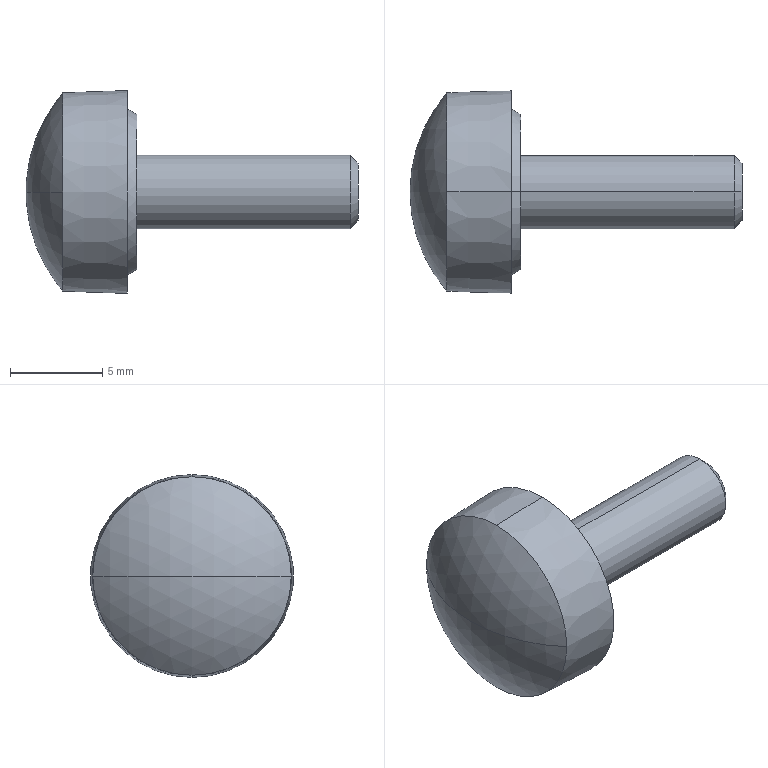Part | SolidWorks | features BaseBody 1 | 1 solid | 13 faces | box 18 x 11 x 11 mm | volume 599.857 mm3 | cone 6 | plane 3 | sphere 2 | cylinder 2 | commonest cylinder face diameters 4 x2
STEP:
#1=CARTESIAN_POINT('',(-4.,5.378,0.));
#2=VERTEX_POINT('',#1);
#3=CARTESIAN_POINT('',(-4.,-5.378,0.));
#4=VERTEX_POINT('',#3);
#5=CARTESIAN_POINT('',(2.23,0.,0.));
#6=DIRECTION('',(0.,0.,1.));
#7=DIRECTION('',(-0.757,0.6534,0.));
#8=AXIS2_PLACEMENT_3D('',#5,#6,#7);
#9=CIRCLE('',#8,8.23);
#10=EDGE_CURVE('',#2,#4,#9,.T.);
#11=ORIENTED_EDGE('',*,*,#10,.F.);
#12=CARTESIAN_POINT('',(-4.,0.,-5.378));
#13=VERTEX_POINT('',#12);
#14=CARTESIAN_POINT('',(-4.,0.,0.));
#15=DIRECTION('',(1.,0.,0.));
#16=DIRECTION('',(0.,0.,-1.));
#17=AXIS2_PLACEMENT_3D('',#14,#15,#16);
#18=CIRCLE('',#17,5.378);
#19=EDGE_CURVE('',#13,#2,#18,.T.);
#20=ORIENTED_EDGE('',*,*,#19,.F.);
#21=CARTESIAN_POINT('',(-4.,0.,0.));
#22=DIRECTION('',(1.,0.,0.));
#23=DIRECTION('',(0.,0.,-1.));
#24=AXIS2_PLACEMENT_3D('',#21,#22,#23);
#25=CIRCLE('',#24,5.378);
#26=EDGE_CURVE('',#4,#13,#25,.T.);
#27=ORIENTED_EDGE('',*,*,#26,.F.);
#28=EDGE_LOOP('',(#11,#20,#27));
#29=FACE_OUTER_BOUND('',#28,.T.);
#30=CARTESIAN_POINT('',(2.23,0.,0.));
#31=DIRECTION('',(0.,-1.,0.));
#32=DIRECTION('',(0.,0.,1.));
#33=AXIS2_PLACEMENT_3D('',#30,#31,#32);
#34=SPHERICAL_SURFACE('',#33,8.23);
#35=ADVANCED_FACE('',(#29),#34,.T.);
#36=ORIENTED_EDGE('',*,*,#10,.T.);
#37=CARTESIAN_POINT('',(-4.,0.,5.378));
#38=VERTEX_POINT('',#37);
#39=CARTESIAN_POINT('',(-4.,0.,0.));
#40=DIRECTION('',(1.,0.,0.));
#41=DIRECTION('',(0.,0.,-1.));
#42=AXIS2_PLACEMENT_3D('',#39,#40,#41);
#43=CIRCLE('',#42,5.378);
#44=EDGE_CURVE('',#38,#4,#43,.T.);
#45=ORIENTED_EDGE('',*,*,#44,.F.);
#46=CARTESIAN_POINT('',(-4.,0.,0.));
#47=DIRECTION('',(1.,0.,0.));
#48=DIRECTION('',(0.,0.,-1.));
#49=AXIS2_PLACEMENT_3D('',#46,#47,#48);
#50=CIRCLE('',#49,5.378);
#51=EDGE_CURVE('',#2,#38,#50,.T.);
#52=ORIENTED_EDGE('',*,*,#51,.F.);
#53=EDGE_LOOP('',(#36,#45,#52));
#54=FACE_OUTER_BOUND('',#53,.T.);
#55=CARTESIAN_POINT('',(2.23,0.,0.));
#56=DIRECTION('',(0.,1.,0.));
#57=DIRECTION('',(0.,0.,-1.));
#58=AXIS2_PLACEMENT_3D('',#55,#56,#57);
#59=SPHERICAL_SURFACE('',#58,8.23);
#60=ADVANCED_FACE('',(#54),#59,.T.);
#61=CARTESIAN_POINT('',(-0.5,0.,5.5));
#62=VERTEX_POINT('',#61);
#63=CARTESIAN_POINT('',(-4.,0.,5.378));
#64=DIRECTION('',(0.9994,0.,0.0349));
#65=VECTOR('',#64,1000.);
#66=LINE('',#63,#65);
#67=EDGE_CURVE('',#38,#62,#66,.T.);
#68=ORIENTED_EDGE('',*,*,#67,.T.);
#69=CARTESIAN_POINT('',(-0.5,0.,-5.5));
#70=VERTEX_POINT('',#69);
#71=CARTESIAN_POINT('',(-0.5,0.,0.));
#72=DIRECTION('',(1.,0.,0.));
#73=DIRECTION('',(0.,0.,-1.));
#74=AXIS2_PLACEMENT_3D('',#71,#72,#73);
#75=CIRCLE('',#74,5.5);
#76=EDGE_CURVE('',#70,#62,#75,.T.);
#77=ORIENTED_EDGE('',*,*,#76,.F.);
#78=CARTESIAN_POINT('',(-4.,0.,-5.378));
#79=DIRECTION('',(0.9994,0.,-0.0349));
#80=VECTOR('',#79,1000.);
#81=LINE('',#78,#80);
#82=EDGE_CURVE('',#13,#70,#81,.T.);
#83=ORIENTED_EDGE('',*,*,#82,.F.);
#84=ORIENTED_EDGE('',*,*,#19,.T.);
#85=ORIENTED_EDGE('',*,*,#51,.T.);
#86=EDGE_LOOP('',(#68,#77,#83,#84,#85));
#87=FACE_OUTER_BOUND('',#86,.T.);
#88=CARTESIAN_POINT('',(-4.,0.,0.));
#89=DIRECTION('',(1.,0.,0.));
#90=DIRECTION('',(0.,-1.,0.));
#91=AXIS2_PLACEMENT_3D('',#88,#89,#90);
#92=CONICAL_SURFACE('',#91,5.378,0.03491);
#93=ADVANCED_FACE('',(#87),#92,.T.);
#94=ORIENTED_EDGE('',*,*,#67,.F.);
#95=ORIENTED_EDGE('',*,*,#44,.T.);
#96=ORIENTED_EDGE('',*,*,#26,.T.);
#97=ORIENTED_EDGE('',*,*,#82,.T.);
#98=CARTESIAN_POINT('',(-0.5,0.,0.));
#99=DIRECTION('',(1.,0.,0.));
#100=DIRECTION('',(0.,0.,-1.));
#101=AXIS2_PLACEMENT_3D('',#98,#99,#100);
#102=CIRCLE('',#101,5.5);
#103=EDGE_CURVE('',#62,#70,#102,.T.);
#104=ORIENTED_EDGE('',*,*,#103,.F.);
#105=EDGE_LOOP('',(#94,#95,#96,#97,#104));
#106=FACE_OUTER_BOUND('',#105,.T.);
#107=CARTESIAN_POINT('',(-4.,0.,0.));
#108=DIRECTION('',(1.,0.,0.));
#109=DIRECTION('',(0.,1.,0.));
#110=AXIS2_PLACEMENT_3D('',#107,#108,#109);
#111=CONICAL_SURFACE('',#110,5.378,0.03491);
#112=ADVANCED_FACE('',(#106),#111,.T.);
#113=CARTESIAN_POINT('',(-0.5,0.,4.5));
#114=VERTEX_POINT('',#113);
#115=CARTESIAN_POINT('',(-0.5,0.,-4.5));
#116=VERTEX_POINT('',#115);
#117=CARTESIAN_POINT('',(-0.5,0.,0.));
#118=DIRECTION('',(1.,0.,0.));
#119=DIRECTION('',(0.,0.,-1.));
#120=AXIS2_PLACEMENT_3D('',#117,#118,#119);
#121=CIRCLE('',#120,4.5);
#122=EDGE_CURVE('',#114,#116,#121,.T.);
#123=ORIENTED_EDGE('',*,*,#122,.F.);
#124=CARTESIAN_POINT('',(-0.5,0.,0.));
#125=DIRECTION('',(1.,0.,0.));
#126=DIRECTION('',(0.,0.,-1.));
#127=AXIS2_PLACEMENT_3D('',#124,#125,#126);
#128=CIRCLE('',#127,4.5);
#129=EDGE_CURVE('',#116,#114,#128,.T.);
#130=ORIENTED_EDGE('',*,*,#129,.F.);
#131=EDGE_LOOP('',(#123,#130));
#132=FACE_BOUND('',#131,.T.);
#133=ORIENTED_EDGE('',*,*,#76,.T.);
#134=ORIENTED_EDGE('',*,*,#103,.T.);
#135=EDGE_LOOP('',(#133,#134));
#136=FACE_OUTER_BOUND('',#135,.T.);
#137=CARTESIAN_POINT('',(-0.5,5.5,0.));
#138=DIRECTION('',(-1.,0.,0.));
#139=DIRECTION('',(0.,0.,1.));
#140=AXIS2_PLACEMENT_3D('',#137,#138,#139);
#141=PLANE('',#140);
#142=ADVANCED_FACE('',(#132,#136),#141,.F.);
#143=CARTESIAN_POINT('',(0.,0.,-4.211));
#144=VERTEX_POINT('',#143);
#145=CARTESIAN_POINT('',(0.,0.,-4.211));
#146=DIRECTION('',(-0.866,0.,-0.5));
#147=VECTOR('',#146,1000.);
#148=LINE('',#145,#147);
#149=EDGE_CURVE('',#144,#116,#148,.T.);
#150=ORIENTED_EDGE('',*,*,#149,.T.);
#151=ORIENTED_EDGE('',*,*,#129,.T.);
#152=CARTESIAN_POINT('',(0.,0.,4.211));
#153=VERTEX_POINT('',#152);
#154=CARTESIAN_POINT('',(0.,0.,4.211));
#155=DIRECTION('',(-0.866,0.,0.5));
#156=VECTOR('',#155,1000.);
#157=LINE('',#154,#156);
#158=EDGE_CURVE('',#153,#114,#157,.T.);
#159=ORIENTED_EDGE('',*,*,#158,.F.);
#160=CARTESIAN_POINT('',(0.,0.,0.));
#161=DIRECTION('',(1.,0.,0.));
#162=DIRECTION('',(0.,0.,-1.));
#163=AXIS2_PLACEMENT_3D('',#160,#161,#162);
#164=CIRCLE('',#163,4.211);
#165=EDGE_CURVE('',#144,#153,#164,.T.);
#166=ORIENTED_EDGE('',*,*,#165,.F.);
#167=EDGE_LOOP('',(#150,#151,#159,#166));
#168=FACE_OUTER_BOUND('',#167,.T.);
#169=CARTESIAN_POINT('',(-0.5,0.,0.));
#170=DIRECTION('',(-1.,0.,0.));
#171=DIRECTION('',(0.,-1.,0.));
#172=AXIS2_PLACEMENT_3D('',#169,#170,#171);
#173=CONICAL_SURFACE('',#172,4.5,0.5236);
#174=ADVANCED_FACE('',(#168),#173,.T.);
#175=CARTESIAN_POINT('',(0.,0.,2.));
#176=VERTEX_POINT('',#175);
#177=CARTESIAN_POINT('',(0.,0.,-2.));
#178=VERTEX_POINT('',#177);
#179=CARTESIAN_POINT('',(0.,0.,0.));
#180=DIRECTION('',(1.,0.,0.));
#181=DIRECTION('',(0.,0.,-1.));
#182=AXIS2_PLACEMENT_3D('',#179,#180,#181);
#183=CIRCLE('',#182,2.);
#184=EDGE_CURVE('',#176,#178,#183,.T.);
#185=ORIENTED_EDGE('',*,*,#184,.F.);
#186=CARTESIAN_POINT('',(0.,0.,0.));
#187=DIRECTION('',(1.,0.,0.));
#188=DIRECTION('',(0.,0.,-1.));
#189=AXIS2_PLACEMENT_3D('',#186,#187,#188);
#190=CIRCLE('',#189,2.);
#191=EDGE_CURVE('',#178,#176,#190,.T.);
#192=ORIENTED_EDGE('',*,*,#191,.F.);
#193=EDGE_LOOP('',(#185,#192));
#194=FACE_BOUND('',#193,.T.);
#195=ORIENTED_EDGE('',*,*,#165,.T.);
#196=CARTESIAN_POINT('',(0.,0.,0.));
#197=DIRECTION('',(1.,0.,0.));
#198=DIRECTION('',(0.,0.,-1.));
#199=AXIS2_PLACEMENT_3D('',#196,#197,#198);
#200=CIRCLE('',#199,4.211);
#201=EDGE_CURVE('',#153,#144,#200,.T.);
#202=ORIENTED_EDGE('',*,*,#201,.T.);
#203=EDGE_LOOP('',(#195,#202));
#204=FACE_OUTER_BOUND('',#203,.T.);
#205=CARTESIAN_POINT('',(0.,4.211,0.));
#206=DIRECTION('',(-1.,0.,0.));
#207=DIRECTION('',(0.,0.,1.));
#208=AXIS2_PLACEMENT_3D('',#205,#206,#207);
#209=PLANE('',#208);
#210=ADVANCED_FACE('',(#194,#204),#209,.F.);
#211=ORIENTED_EDGE('',*,*,#149,.F.);
#212=ORIENTED_EDGE('',*,*,#201,.F.);
#213=ORIENTED_EDGE('',*,*,#158,.T.);
#214=ORIENTED_EDGE('',*,*,#122,.T.);
#215=EDGE_LOOP('',(#211,#212,#213,#214));
#216=FACE_OUTER_BOUND('',#215,.T.);
#217=CARTESIAN_POINT('',(-0.5,0.,0.));
#218=DIRECTION('',(-1.,0.,0.));
#219=DIRECTION('',(0.,1.,0.));
#220=AXIS2_PLACEMENT_3D('',#217,#218,#219);
#221=CONICAL_SURFACE('',#220,4.5,0.5236);
#222=ADVANCED_FACE('',(#216),#221,.T.);
#223=CARTESIAN_POINT('',(11.571,0.,2.));
#224=VERTEX_POINT('',#223);
#225=CARTESIAN_POINT('',(0.,0.,2.));
#226=DIRECTION('',(1.,0.,0.));
#227=VECTOR('',#226,1000.);
#228=LINE('',#225,#227);
#229=EDGE_CURVE('',#176,#224,#228,.T.);
#230=ORIENTED_EDGE('',*,*,#229,.T.);
#231=CARTESIAN_POINT('',(11.571,0.,-2.));
#232=VERTEX_POINT('',#231);
#233=CARTESIAN_POINT('',(11.571,0.,0.));
#234=DIRECTION('',(1.,0.,0.));
#235=DIRECTION('',(0.,0.,-1.));
#236=AXIS2_PLACEMENT_3D('',#233,#234,#235);
#237=CIRCLE('',#236,2.);
#238=EDGE_CURVE('',#232,#224,#237,.T.);
#239=ORIENTED_EDGE('',*,*,#238,.F.);
#240=CARTESIAN_POINT('',(0.,0.,-2.));
#241=DIRECTION('',(1.,0.,0.));
#242=VECTOR('',#241,1000.);
#243=LINE('',#240,#242);
#244=EDGE_CURVE('',#178,#232,#243,.T.);
#245=ORIENTED_EDGE('',*,*,#244,.F.);
#246=ORIENTED_EDGE('',*,*,#191,.T.);
#247=EDGE_LOOP('',(#230,#239,#245,#246));
#248=FACE_OUTER_BOUND('',#247,.T.);
#249=CARTESIAN_POINT('',(12.,0.,0.));
#250=DIRECTION('',(1.,0.,0.));
#251=DIRECTION('',(0.,-1.,0.));
#252=AXIS2_PLACEMENT_3D('',#249,#250,#251);
#253=CYLINDRICAL_SURFACE('',#252,2.);
#254=ADVANCED_FACE('',(#248),#253,.T.);
#255=ORIENTED_EDGE('',*,*,#229,.F.);
#256=ORIENTED_EDGE('',*,*,#184,.T.);
#257=ORIENTED_EDGE('',*,*,#244,.T.);
#258=CARTESIAN_POINT('',(11.571,0.,0.));
#259=DIRECTION('',(1.,0.,0.));
#260=DIRECTION('',(0.,0.,-1.));
#261=AXIS2_PLACEMENT_3D('',#258,#259,#260);
#262=CIRCLE('',#261,2.);
#263=EDGE_CURVE('',#224,#232,#262,.T.);
#264=ORIENTED_EDGE('',*,*,#263,.F.);
#265=EDGE_LOOP('',(#255,#256,#257,#264));
#266=FACE_OUTER_BOUND('',#265,.T.);
#267=CARTESIAN_POINT('',(12.,0.,0.));
#268=DIRECTION('',(1.,0.,0.));
#269=DIRECTION('',(0.,1.,0.));
#270=AXIS2_PLACEMENT_3D('',#267,#268,#269);
#271=CYLINDRICAL_SURFACE('',#270,2.);
#272=ADVANCED_FACE('',(#266),#271,.T.);
#273=CARTESIAN_POINT('',(12.,0.,-1.57));
#274=VERTEX_POINT('',#273);
#275=CARTESIAN_POINT('',(12.,0.,-1.57));
#276=DIRECTION('',(-0.7071,0.,-0.7071));
#277=VECTOR('',#276,1000.);
#278=LINE('',#275,#277);
#279=EDGE_CURVE('',#274,#232,#278,.T.);
#280=ORIENTED_EDGE('',*,*,#279,.F.);
#281=CARTESIAN_POINT('',(12.,0.,1.57));
#282=VERTEX_POINT('',#281);
#283=CARTESIAN_POINT('',(12.,0.,0.));
#284=DIRECTION('',(1.,0.,0.));
#285=DIRECTION('',(0.,0.,-1.));
#286=AXIS2_PLACEMENT_3D('',#283,#284,#285);
#287=CIRCLE('',#286,1.571);
#288=EDGE_CURVE('',#282,#274,#287,.T.);
#289=ORIENTED_EDGE('',*,*,#288,.F.);
#290=CARTESIAN_POINT('',(12.,0.,1.57));
#291=DIRECTION('',(-0.7071,0.,0.7071));
#292=VECTOR('',#291,1000.);
#293=LINE('',#290,#292);
#294=EDGE_CURVE('',#282,#224,#293,.T.);
#295=ORIENTED_EDGE('',*,*,#294,.T.);
#296=ORIENTED_EDGE('',*,*,#263,.T.);
#297=EDGE_LOOP('',(#280,#289,#295,#296));
#298=FACE_OUTER_BOUND('',#297,.T.);
#299=CARTESIAN_POINT('',(11.571,0.,0.));
#300=DIRECTION('',(-1.,0.,0.));
#301=DIRECTION('',(0.,1.,0.));
#302=AXIS2_PLACEMENT_3D('',#299,#300,#301);
#303=CONICAL_SURFACE('',#302,2.,0.7854);
#304=ADVANCED_FACE('',(#298),#303,.T.);
#305=ORIENTED_EDGE('',*,*,#279,.T.);
#306=ORIENTED_EDGE('',*,*,#238,.T.);
#307=ORIENTED_EDGE('',*,*,#294,.F.);
#308=CARTESIAN_POINT('',(12.,0.,0.));
#309=DIRECTION('',(1.,0.,0.));
#310=DIRECTION('',(0.,0.,-1.));
#311=AXIS2_PLACEMENT_3D('',#308,#309,#310);
#312=CIRCLE('',#311,1.571);
#313=EDGE_CURVE('',#274,#282,#312,.T.);
#314=ORIENTED_EDGE('',*,*,#313,.F.);
#315=EDGE_LOOP('',(#305,#306,#307,#314));
#316=FACE_OUTER_BOUND('',#315,.T.);
#317=CARTESIAN_POINT('',(11.571,0.,0.));
#318=DIRECTION('',(-1.,0.,0.));
#319=DIRECTION('',(0.,-1.,0.));
#320=AXIS2_PLACEMENT_3D('',#317,#318,#319);
#321=CONICAL_SURFACE('',#320,2.,0.7854);
#322=ADVANCED_FACE('',(#316),#321,.T.);
#323=ORIENTED_EDGE('',*,*,#313,.T.);
#324=ORIENTED_EDGE('',*,*,#288,.T.);
#325=EDGE_LOOP('',(#323,#324));
#326=FACE_OUTER_BOUND('',#325,.T.);
#327=CARTESIAN_POINT('',(12.,1.571,0.));
#328=DIRECTION('',(-1.,0.,0.));
#329=DIRECTION('',(0.,0.,1.));
#330=AXIS2_PLACEMENT_3D('',#327,#328,#329);
#331=PLANE('',#330);
#332=ADVANCED_FACE('',(#326),#331,.F.);
#333=CLOSED_SHELL('',(#35,#60,#93,#112,#142,#174,#210,#222,#254,#272,#304,#322,#332));
#334=MANIFOLD_SOLID_BREP('',#333);
#335=CARTESIAN_POINT('',(0.,0.,0.));
#336=DIRECTION('',(0.,0.,1.));
#337=DIRECTION('',(1.,0.,0.));
#338=AXIS2_PLACEMENT_3D('',#335,#336,#337);
#339=(LENGTH_UNIT()NAMED_UNIT(*)SI_UNIT(.MILLI.,.METRE.));
#340=UNCERTAINTY_MEASURE_WITH_UNIT(LENGTH_MEASURE(0.00001),#339,'','');
#341=(NAMED_UNIT(*)PLANE_ANGLE_UNIT()SI_UNIT($,.RADIAN.));
#342=(NAMED_UNIT(*)SI_UNIT($,.STERADIAN.)SOLID_ANGLE_UNIT());
#343=(GEOMETRIC_REPRESENTATION_CONTEXT(3)GLOBAL_UNCERTAINTY_ASSIGNED_CONTEXT((#340))GLOBAL_UNIT_ASSIGNED_CONTEXT((#339,#341,#342))REPRESENTATION_CONTEXT('',''));
#344=ADVANCED_BREP_SHAPE_REPRESENTATION('',(#334,#338),#343);